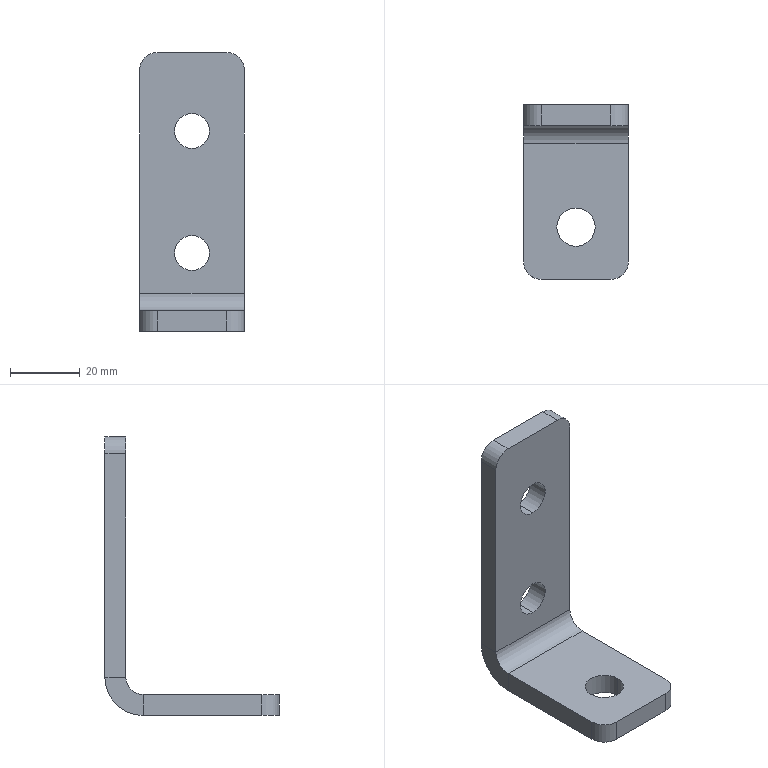Part | STEP file | SYL_0392D6J1SYL0380DJ100-808646 | 1 solid | 24 faces | box 30 x 50 x 80 mm | volume 20061 mm3 | cylinder 12 | plane 12 | commonest cylinder face diameters 10 x9 11 x2 22 x1
STEP:
#1=CARTESIAN_POINT('',(0.,25.,27.5));
#2=VERTEX_POINT('',#1);
#3=CARTESIAN_POINT('',(0.,19.,27.5));
#4=VERTEX_POINT('',#3);
#5=CARTESIAN_POINT('',(0.,19.,27.5));
#6=DIRECTION('',(0.,-1.,0.));
#7=VECTOR('',#6,1000.);
#8=LINE('',#5,#7);
#9=EDGE_CURVE('',#2,#4,#8,.T.);
#10=ORIENTED_EDGE('',*,*,#9,.F.);
#11=CARTESIAN_POINT('',(0.,25.,17.5));
#12=VERTEX_POINT('',#11);
#13=CARTESIAN_POINT('',(0.,25.,22.5));
#14=DIRECTION('',(0.,1.,0.));
#15=DIRECTION('',(0.,0.,1.));
#16=AXIS2_PLACEMENT_3D('',#13,#14,#15);
#17=CIRCLE('',#16,5.);
#18=EDGE_CURVE('',#2,#12,#17,.T.);
#19=ORIENTED_EDGE('',*,*,#18,.T.);
#20=CARTESIAN_POINT('',(0.,19.,17.5));
#21=VERTEX_POINT('',#20);
#22=CARTESIAN_POINT('',(0.,19.,17.5));
#23=DIRECTION('',(0.,-1.,0.));
#24=VECTOR('',#23,1000.);
#25=LINE('',#22,#24);
#26=EDGE_CURVE('',#12,#21,#25,.T.);
#27=ORIENTED_EDGE('',*,*,#26,.T.);
#28=CARTESIAN_POINT('',(0.,19.,22.5));
#29=DIRECTION('',(0.,1.,0.));
#30=DIRECTION('',(0.,0.,1.));
#31=AXIS2_PLACEMENT_3D('',#28,#29,#30);
#32=CIRCLE('',#31,5.);
#33=EDGE_CURVE('',#4,#21,#32,.T.);
#34=ORIENTED_EDGE('',*,*,#33,.F.);
#35=EDGE_LOOP('',(#10,#19,#27,#34));
#36=FACE_OUTER_BOUND('',#35,.T.);
#37=CARTESIAN_POINT('',(0.,19.,22.5));
#38=DIRECTION('',(0.,-1.,0.));
#39=DIRECTION('',(0.,0.,-1.));
#40=AXIS2_PLACEMENT_3D('',#37,#38,#39);
#41=CYLINDRICAL_SURFACE('',#40,5.);
#42=ADVANCED_FACE('',(#36),#41,.F.);
#43=CARTESIAN_POINT('',(0.,25.,62.5));
#44=VERTEX_POINT('',#43);
#45=CARTESIAN_POINT('',(0.,19.,62.5));
#46=VERTEX_POINT('',#45);
#47=CARTESIAN_POINT('',(0.,19.,62.5));
#48=DIRECTION('',(0.,-1.,0.));
#49=VECTOR('',#48,1000.);
#50=LINE('',#47,#49);
#51=EDGE_CURVE('',#44,#46,#50,.T.);
#52=ORIENTED_EDGE('',*,*,#51,.F.);
#53=CARTESIAN_POINT('',(0.,25.,52.5));
#54=VERTEX_POINT('',#53);
#55=CARTESIAN_POINT('',(0.,25.,57.5));
#56=DIRECTION('',(0.,1.,0.));
#57=DIRECTION('',(0.,0.,1.));
#58=AXIS2_PLACEMENT_3D('',#55,#56,#57);
#59=CIRCLE('',#58,5.);
#60=EDGE_CURVE('',#44,#54,#59,.T.);
#61=ORIENTED_EDGE('',*,*,#60,.T.);
#62=CARTESIAN_POINT('',(0.,19.,52.5));
#63=VERTEX_POINT('',#62);
#64=CARTESIAN_POINT('',(0.,19.,52.5));
#65=DIRECTION('',(0.,-1.,0.));
#66=VECTOR('',#65,1000.);
#67=LINE('',#64,#66);
#68=EDGE_CURVE('',#54,#63,#67,.T.);
#69=ORIENTED_EDGE('',*,*,#68,.T.);
#70=CARTESIAN_POINT('',(0.,19.,57.5));
#71=DIRECTION('',(0.,1.,0.));
#72=DIRECTION('',(0.,0.,1.));
#73=AXIS2_PLACEMENT_3D('',#70,#71,#72);
#74=CIRCLE('',#73,5.);
#75=EDGE_CURVE('',#46,#63,#74,.T.);
#76=ORIENTED_EDGE('',*,*,#75,.F.);
#77=EDGE_LOOP('',(#52,#61,#69,#76));
#78=FACE_OUTER_BOUND('',#77,.T.);
#79=CARTESIAN_POINT('',(0.,19.,57.5));
#80=DIRECTION('',(0.,-1.,0.));
#81=DIRECTION('',(0.,0.,-1.));
#82=AXIS2_PLACEMENT_3D('',#79,#80,#81);
#83=CYLINDRICAL_SURFACE('',#82,5.);
#84=ADVANCED_FACE('',(#78),#83,.F.);
#85=CARTESIAN_POINT('',(5.5,-10.,0.));
#86=VERTEX_POINT('',#85);
#87=CARTESIAN_POINT('',(5.5,-10.,6.));
#88=VERTEX_POINT('',#87);
#89=CARTESIAN_POINT('',(5.5,-10.,6.));
#90=DIRECTION('',(0.,0.,1.));
#91=VECTOR('',#90,1000.);
#92=LINE('',#89,#91);
#93=EDGE_CURVE('',#86,#88,#92,.T.);
#94=ORIENTED_EDGE('',*,*,#93,.F.);
#95=CARTESIAN_POINT('',(-5.5,-10.,0.));
#96=VERTEX_POINT('',#95);
#97=CARTESIAN_POINT('',(0.,-10.,0.));
#98=DIRECTION('',(0.,0.,-1.));
#99=DIRECTION('',(-1.,0.,0.));
#100=AXIS2_PLACEMENT_3D('',#97,#98,#99);
#101=CIRCLE('',#100,5.5);
#102=EDGE_CURVE('',#86,#96,#101,.T.);
#103=ORIENTED_EDGE('',*,*,#102,.T.);
#104=CARTESIAN_POINT('',(-5.5,-10.,6.));
#105=VERTEX_POINT('',#104);
#106=CARTESIAN_POINT('',(-5.5,-10.,6.));
#107=DIRECTION('',(0.,0.,1.));
#108=VECTOR('',#107,1000.);
#109=LINE('',#106,#108);
#110=EDGE_CURVE('',#96,#105,#109,.T.);
#111=ORIENTED_EDGE('',*,*,#110,.T.);
#112=CARTESIAN_POINT('',(0.,-10.,6.));
#113=DIRECTION('',(0.,0.,-1.));
#114=DIRECTION('',(1.,0.,0.));
#115=AXIS2_PLACEMENT_3D('',#112,#113,#114);
#116=CIRCLE('',#115,5.5);
#117=EDGE_CURVE('',#88,#105,#116,.T.);
#118=ORIENTED_EDGE('',*,*,#117,.F.);
#119=EDGE_LOOP('',(#94,#103,#111,#118));
#120=FACE_OUTER_BOUND('',#119,.T.);
#121=CARTESIAN_POINT('',(0.,-10.,6.));
#122=DIRECTION('',(0.,0.,1.));
#123=DIRECTION('',(1.,0.,0.));
#124=AXIS2_PLACEMENT_3D('',#121,#122,#123);
#125=CYLINDRICAL_SURFACE('',#124,5.5);
#126=ADVANCED_FACE('',(#120),#125,.F.);
#127=CARTESIAN_POINT('',(15.,25.,75.));
#128=VERTEX_POINT('',#127);
#129=CARTESIAN_POINT('',(15.,19.,75.));
#130=VERTEX_POINT('',#129);
#131=CARTESIAN_POINT('',(15.,19.,75.));
#132=DIRECTION('',(0.,-1.,0.));
#133=VECTOR('',#132,1000.);
#134=LINE('',#131,#133);
#135=EDGE_CURVE('',#128,#130,#134,.T.);
#136=ORIENTED_EDGE('',*,*,#135,.F.);
#137=CARTESIAN_POINT('',(10.,25.,80.));
#138=VERTEX_POINT('',#137);
#139=CARTESIAN_POINT('',(10.,25.,75.));
#140=DIRECTION('',(0.,-1.,0.));
#141=DIRECTION('',(0.,0.,-1.));
#142=AXIS2_PLACEMENT_3D('',#139,#140,#141);
#143=CIRCLE('',#142,5.);
#144=EDGE_CURVE('',#128,#138,#143,.T.);
#145=ORIENTED_EDGE('',*,*,#144,.T.);
#146=CARTESIAN_POINT('',(10.,19.,80.));
#147=VERTEX_POINT('',#146);
#148=CARTESIAN_POINT('',(10.,19.,80.));
#149=DIRECTION('',(0.,-1.,0.));
#150=VECTOR('',#149,1000.);
#151=LINE('',#148,#150);
#152=EDGE_CURVE('',#138,#147,#151,.T.);
#153=ORIENTED_EDGE('',*,*,#152,.T.);
#154=CARTESIAN_POINT('',(10.,19.,75.));
#155=DIRECTION('',(0.,-1.,0.));
#156=DIRECTION('',(1.,0.,0.));
#157=AXIS2_PLACEMENT_3D('',#154,#155,#156);
#158=CIRCLE('',#157,5.);
#159=EDGE_CURVE('',#130,#147,#158,.T.);
#160=ORIENTED_EDGE('',*,*,#159,.F.);
#161=EDGE_LOOP('',(#136,#145,#153,#160));
#162=FACE_OUTER_BOUND('',#161,.T.);
#163=CARTESIAN_POINT('',(10.,19.,75.));
#164=DIRECTION('',(0.,-1.,0.));
#165=DIRECTION('',(0.,0.,-1.));
#166=AXIS2_PLACEMENT_3D('',#163,#164,#165);
#167=CYLINDRICAL_SURFACE('',#166,5.);
#168=ADVANCED_FACE('',(#162),#167,.T.);
#169=ORIENTED_EDGE('',*,*,#152,.F.);
#170=CARTESIAN_POINT('',(-10.,25.,80.));
#171=VERTEX_POINT('',#170);
#172=CARTESIAN_POINT('',(7.872,25.,80.));
#173=DIRECTION('',(1.,0.,0.));
#174=VECTOR('',#173,1000.);
#175=LINE('',#172,#174);
#176=EDGE_CURVE('',#171,#138,#175,.T.);
#177=ORIENTED_EDGE('',*,*,#176,.F.);
#178=CARTESIAN_POINT('',(-10.,19.,80.));
#179=VERTEX_POINT('',#178);
#180=CARTESIAN_POINT('',(-10.,19.,80.));
#181=DIRECTION('',(0.,-1.,0.));
#182=VECTOR('',#181,1000.);
#183=LINE('',#180,#182);
#184=EDGE_CURVE('',#171,#179,#183,.T.);
#185=ORIENTED_EDGE('',*,*,#184,.T.);
#186=CARTESIAN_POINT('',(-10.,19.,80.));
#187=DIRECTION('',(1.,0.,0.));
#188=VECTOR('',#187,1000.);
#189=LINE('',#186,#188);
#190=EDGE_CURVE('',#179,#147,#189,.T.);
#191=ORIENTED_EDGE('',*,*,#190,.T.);
#192=EDGE_LOOP('',(#169,#177,#185,#191));
#193=FACE_OUTER_BOUND('',#192,.T.);
#194=CARTESIAN_POINT('',(-10.,19.,80.));
#195=DIRECTION('',(0.,0.,-1.));
#196=DIRECTION('',(1.,0.,0.));
#197=AXIS2_PLACEMENT_3D('',#194,#195,#196);
#198=PLANE('',#197);
#199=ADVANCED_FACE('',(#193),#198,.F.);
#200=ORIENTED_EDGE('',*,*,#184,.F.);
#201=CARTESIAN_POINT('',(-15.,25.,75.));
#202=VERTEX_POINT('',#201);
#203=CARTESIAN_POINT('',(-10.,25.,75.));
#204=DIRECTION('',(0.,-1.,0.));
#205=DIRECTION('',(0.,0.,-1.));
#206=AXIS2_PLACEMENT_3D('',#203,#204,#205);
#207=CIRCLE('',#206,5.);
#208=EDGE_CURVE('',#171,#202,#207,.T.);
#209=ORIENTED_EDGE('',*,*,#208,.T.);
#210=CARTESIAN_POINT('',(-15.,19.,75.));
#211=VERTEX_POINT('',#210);
#212=CARTESIAN_POINT('',(-15.,19.,75.));
#213=DIRECTION('',(0.,-1.,0.));
#214=VECTOR('',#213,1000.);
#215=LINE('',#212,#214);
#216=EDGE_CURVE('',#202,#211,#215,.T.);
#217=ORIENTED_EDGE('',*,*,#216,.T.);
#218=CARTESIAN_POINT('',(-10.,19.,75.));
#219=DIRECTION('',(0.,-1.,0.));
#220=DIRECTION('',(0.,0.,1.));
#221=AXIS2_PLACEMENT_3D('',#218,#219,#220);
#222=CIRCLE('',#221,5.);
#223=EDGE_CURVE('',#179,#211,#222,.T.);
#224=ORIENTED_EDGE('',*,*,#223,.F.);
#225=EDGE_LOOP('',(#200,#209,#217,#224));
#226=FACE_OUTER_BOUND('',#225,.T.);
#227=CARTESIAN_POINT('',(-10.,19.,75.));
#228=DIRECTION('',(0.,-1.,0.));
#229=DIRECTION('',(0.,0.,-1.));
#230=AXIS2_PLACEMENT_3D('',#227,#228,#229);
#231=CYLINDRICAL_SURFACE('',#230,5.);
#232=ADVANCED_FACE('',(#226),#231,.T.);
#233=ORIENTED_EDGE('',*,*,#216,.F.);
#234=CARTESIAN_POINT('',(-15.,25.,11.));
#235=VERTEX_POINT('',#234);
#236=CARTESIAN_POINT('',(-15.,25.,0.));
#237=DIRECTION('',(0.,0.,1.));
#238=VECTOR('',#237,1000.);
#239=LINE('',#236,#238);
#240=EDGE_CURVE('',#235,#202,#239,.T.);
#241=ORIENTED_EDGE('',*,*,#240,.F.);
#242=CARTESIAN_POINT('',(-15.,19.,11.));
#243=VERTEX_POINT('',#242);
#244=CARTESIAN_POINT('',(-15.,19.,11.));
#245=DIRECTION('',(0.,-1.,0.));
#246=VECTOR('',#245,1000.);
#247=LINE('',#244,#246);
#248=EDGE_CURVE('',#235,#243,#247,.T.);
#249=ORIENTED_EDGE('',*,*,#248,.T.);
#250=CARTESIAN_POINT('',(-15.,19.,11.));
#251=DIRECTION('',(0.,0.,1.));
#252=VECTOR('',#251,1000.);
#253=LINE('',#250,#252);
#254=EDGE_CURVE('',#243,#211,#253,.T.);
#255=ORIENTED_EDGE('',*,*,#254,.T.);
#256=EDGE_LOOP('',(#233,#241,#249,#255));
#257=FACE_OUTER_BOUND('',#256,.T.);
#258=CARTESIAN_POINT('',(-15.,19.,11.));
#259=DIRECTION('',(1.,0.,0.));
#260=DIRECTION('',(0.,0.,1.));
#261=AXIS2_PLACEMENT_3D('',#258,#259,#260);
#262=PLANE('',#261);
#263=ADVANCED_FACE('',(#257),#262,.F.);
#264=ORIENTED_EDGE('',*,*,#248,.F.);
#265=CARTESIAN_POINT('',(-15.,14.,0.));
#266=VERTEX_POINT('',#265);
#267=CARTESIAN_POINT('',(-15.,14.,11.));
#268=DIRECTION('',(1.,0.,0.));
#269=DIRECTION('',(0.,0.,1.));
#270=AXIS2_PLACEMENT_3D('',#267,#268,#269);
#271=CIRCLE('',#270,11.);
#272=EDGE_CURVE('',#266,#235,#271,.T.);
#273=ORIENTED_EDGE('',*,*,#272,.F.);
#274=CARTESIAN_POINT('',(-15.,14.,6.));
#275=VERTEX_POINT('',#274);
#276=CARTESIAN_POINT('',(-15.,14.,6.));
#277=DIRECTION('',(0.,0.,1.));
#278=VECTOR('',#277,1000.);
#279=LINE('',#276,#278);
#280=EDGE_CURVE('',#266,#275,#279,.T.);
#281=ORIENTED_EDGE('',*,*,#280,.T.);
#282=CARTESIAN_POINT('',(-15.,14.,11.));
#283=DIRECTION('',(1.,0.,0.));
#284=DIRECTION('',(0.,0.,-1.));
#285=AXIS2_PLACEMENT_3D('',#282,#283,#284);
#286=CIRCLE('',#285,5.);
#287=EDGE_CURVE('',#275,#243,#286,.T.);
#288=ORIENTED_EDGE('',*,*,#287,.T.);
#289=EDGE_LOOP('',(#264,#273,#281,#288));
#290=FACE_OUTER_BOUND('',#289,.T.);
#291=CARTESIAN_POINT('',(-15.,14.,11.));
#292=DIRECTION('',(-1.,0.,0.));
#293=DIRECTION('',(0.,0.,1.));
#294=AXIS2_PLACEMENT_3D('',#291,#292,#293);
#295=PLANE('',#294);
#296=ADVANCED_FACE('',(#290),#295,.T.);
#297=ORIENTED_EDGE('',*,*,#280,.F.);
#298=CARTESIAN_POINT('',(-15.,-20.,0.));
#299=VERTEX_POINT('',#298);
#300=CARTESIAN_POINT('',(-15.,0.,0.));
#301=DIRECTION('',(0.,1.,0.));
#302=VECTOR('',#301,1000.);
#303=LINE('',#300,#302);
#304=EDGE_CURVE('',#299,#266,#303,.T.);
#305=ORIENTED_EDGE('',*,*,#304,.F.);
#306=CARTESIAN_POINT('',(-15.,-20.,6.));
#307=VERTEX_POINT('',#306);
#308=CARTESIAN_POINT('',(-15.,-20.,6.));
#309=DIRECTION('',(0.,0.,1.));
#310=VECTOR('',#309,1000.);
#311=LINE('',#308,#310);
#312=EDGE_CURVE('',#299,#307,#311,.T.);
#313=ORIENTED_EDGE('',*,*,#312,.T.);
#314=CARTESIAN_POINT('',(-15.,-20.,6.));
#315=DIRECTION('',(0.,1.,0.));
#316=VECTOR('',#315,1000.);
#317=LINE('',#314,#316);
#318=EDGE_CURVE('',#307,#275,#317,.T.);
#319=ORIENTED_EDGE('',*,*,#318,.T.);
#320=EDGE_LOOP('',(#297,#305,#313,#319));
#321=FACE_OUTER_BOUND('',#320,.T.);
#322=CARTESIAN_POINT('',(-15.,-20.,6.));
#323=DIRECTION('',(1.,0.,0.));
#324=DIRECTION('',(0.,1.,0.));
#325=AXIS2_PLACEMENT_3D('',#322,#323,#324);
#326=PLANE('',#325);
#327=ADVANCED_FACE('',(#321),#326,.F.);
#328=ORIENTED_EDGE('',*,*,#312,.F.);
#329=CARTESIAN_POINT('',(-10.,-25.,0.));
#330=VERTEX_POINT('',#329);
#331=CARTESIAN_POINT('',(-10.,-20.,0.));
#332=DIRECTION('',(0.,0.,1.));
#333=DIRECTION('',(1.,0.,0.));
#334=AXIS2_PLACEMENT_3D('',#331,#332,#333);
#335=CIRCLE('',#334,5.);
#336=EDGE_CURVE('',#299,#330,#335,.T.);
#337=ORIENTED_EDGE('',*,*,#336,.T.);
#338=CARTESIAN_POINT('',(-10.,-25.,6.));
#339=VERTEX_POINT('',#338);
#340=CARTESIAN_POINT('',(-10.,-25.,6.));
#341=DIRECTION('',(0.,0.,1.));
#342=VECTOR('',#341,1000.);
#343=LINE('',#340,#342);
#344=EDGE_CURVE('',#330,#339,#343,.T.);
#345=ORIENTED_EDGE('',*,*,#344,.T.);
#346=CARTESIAN_POINT('',(-10.,-20.,6.));
#347=DIRECTION('',(0.,0.,1.));
#348=DIRECTION('',(-1.,0.,0.));
#349=AXIS2_PLACEMENT_3D('',#346,#347,#348);
#350=CIRCLE('',#349,5.);
#351=EDGE_CURVE('',#307,#339,#350,.T.);
#352=ORIENTED_EDGE('',*,*,#351,.F.);
#353=EDGE_LOOP('',(#328,#337,#345,#352));
#354=FACE_OUTER_BOUND('',#353,.T.);
#355=CARTESIAN_POINT('',(-10.,-20.,6.));
#356=DIRECTION('',(0.,0.,1.));
#357=DIRECTION('',(1.,0.,0.));
#358=AXIS2_PLACEMENT_3D('',#355,#356,#357);
#359=CYLINDRICAL_SURFACE('',#358,5.);
#360=ADVANCED_FACE('',(#354),#359,.T.);
#361=ORIENTED_EDGE('',*,*,#344,.F.);
#362=CARTESIAN_POINT('',(10.,-25.,0.));
#363=VERTEX_POINT('',#362);
#364=CARTESIAN_POINT('',(0.,-25.,0.));
#365=DIRECTION('',(-1.,0.,0.));
#366=VECTOR('',#365,1000.);
#367=LINE('',#364,#366);
#368=EDGE_CURVE('',#363,#330,#367,.T.);
#369=ORIENTED_EDGE('',*,*,#368,.F.);
#370=CARTESIAN_POINT('',(10.,-25.,6.));
#371=VERTEX_POINT('',#370);
#372=CARTESIAN_POINT('',(10.,-25.,6.));
#373=DIRECTION('',(0.,0.,1.));
#374=VECTOR('',#373,1000.);
#375=LINE('',#372,#374);
#376=EDGE_CURVE('',#363,#371,#375,.T.);
#377=ORIENTED_EDGE('',*,*,#376,.T.);
#378=CARTESIAN_POINT('',(10.,-25.,6.));
#379=DIRECTION('',(-1.,0.,0.));
#380=VECTOR('',#379,1000.);
#381=LINE('',#378,#380);
#382=EDGE_CURVE('',#371,#339,#381,.T.);
#383=ORIENTED_EDGE('',*,*,#382,.T.);
#384=EDGE_LOOP('',(#361,#369,#377,#383));
#385=FACE_OUTER_BOUND('',#384,.T.);
#386=CARTESIAN_POINT('',(10.,-25.,6.));
#387=DIRECTION('',(0.,1.,0.));
#388=DIRECTION('',(-1.,0.,0.));
#389=AXIS2_PLACEMENT_3D('',#386,#387,#388);
#390=PLANE('',#389);
#391=ADVANCED_FACE('',(#385),#390,.F.);
#392=ORIENTED_EDGE('',*,*,#376,.F.);
#393=CARTESIAN_POINT('',(15.,-20.,0.));
#394=VERTEX_POINT('',#393);
#395=CARTESIAN_POINT('',(10.,-20.,0.));
#396=DIRECTION('',(0.,0.,1.));
#397=DIRECTION('',(1.,0.,0.));
#398=AXIS2_PLACEMENT_3D('',#395,#396,#397);
#399=CIRCLE('',#398,5.);
#400=EDGE_CURVE('',#363,#394,#399,.T.);
#401=ORIENTED_EDGE('',*,*,#400,.T.);
#402=CARTESIAN_POINT('',(15.,-20.,6.));
#403=VERTEX_POINT('',#402);
#404=CARTESIAN_POINT('',(15.,-20.,6.));
#405=DIRECTION('',(0.,0.,1.));
#406=VECTOR('',#405,1000.);
#407=LINE('',#404,#406);
#408=EDGE_CURVE('',#394,#403,#407,.T.);
#409=ORIENTED_EDGE('',*,*,#408,.T.);
#410=CARTESIAN_POINT('',(10.,-20.,6.));
#411=DIRECTION('',(0.,0.,1.));
#412=DIRECTION('',(0.,-1.,0.));
#413=AXIS2_PLACEMENT_3D('',#410,#411,#412);
#414=CIRCLE('',#413,5.);
#415=EDGE_CURVE('',#371,#403,#414,.T.);
#416=ORIENTED_EDGE('',*,*,#415,.F.);
#417=EDGE_LOOP('',(#392,#401,#409,#416));
#418=FACE_OUTER_BOUND('',#417,.T.);
#419=CARTESIAN_POINT('',(10.,-20.,6.));
#420=DIRECTION('',(0.,0.,1.));
#421=DIRECTION('',(1.,0.,0.));
#422=AXIS2_PLACEMENT_3D('',#419,#420,#421);
#423=CYLINDRICAL_SURFACE('',#422,5.);
#424=ADVANCED_FACE('',(#418),#423,.T.);
#425=ORIENTED_EDGE('',*,*,#408,.F.);
#426=CARTESIAN_POINT('',(15.,14.,0.));
#427=VERTEX_POINT('',#426);
#428=CARTESIAN_POINT('',(15.,0.,0.));
#429=DIRECTION('',(0.,-1.,0.));
#430=VECTOR('',#429,1000.);
#431=LINE('',#428,#430);
#432=EDGE_CURVE('',#427,#394,#431,.T.);
#433=ORIENTED_EDGE('',*,*,#432,.F.);
#434=CARTESIAN_POINT('',(15.,14.,6.));
#435=VERTEX_POINT('',#434);
#436=CARTESIAN_POINT('',(15.,14.,6.));
#437=DIRECTION('',(0.,0.,1.));
#438=VECTOR('',#437,1000.);
#439=LINE('',#436,#438);
#440=EDGE_CURVE('',#427,#435,#439,.T.);
#441=ORIENTED_EDGE('',*,*,#440,.T.);
#442=CARTESIAN_POINT('',(15.,14.,6.));
#443=DIRECTION('',(0.,-1.,0.));
#444=VECTOR('',#443,1000.);
#445=LINE('',#442,#444);
#446=EDGE_CURVE('',#435,#403,#445,.T.);
#447=ORIENTED_EDGE('',*,*,#446,.T.);
#448=EDGE_LOOP('',(#425,#433,#441,#447));
#449=FACE_OUTER_BOUND('',#448,.T.);
#450=CARTESIAN_POINT('',(15.,14.,6.));
#451=DIRECTION('',(-1.,0.,0.));
#452=DIRECTION('',(0.,-1.,0.));
#453=AXIS2_PLACEMENT_3D('',#450,#451,#452);
#454=PLANE('',#453);
#455=ADVANCED_FACE('',(#449),#454,.F.);
#456=ORIENTED_EDGE('',*,*,#440,.F.);
#457=CARTESIAN_POINT('',(15.,25.,11.));
#458=VERTEX_POINT('',#457);
#459=CARTESIAN_POINT('',(15.,14.,11.));
#460=DIRECTION('',(-1.,0.,0.));
#461=DIRECTION('',(0.,0.,1.));
#462=AXIS2_PLACEMENT_3D('',#459,#460,#461);
#463=CIRCLE('',#462,11.);
#464=EDGE_CURVE('',#458,#427,#463,.T.);
#465=ORIENTED_EDGE('',*,*,#464,.F.);
#466=CARTESIAN_POINT('',(15.,19.,11.));
#467=VERTEX_POINT('',#466);
#468=CARTESIAN_POINT('',(15.,19.,11.));
#469=DIRECTION('',(0.,-1.,0.));
#470=VECTOR('',#469,1000.);
#471=LINE('',#468,#470);
#472=EDGE_CURVE('',#458,#467,#471,.T.);
#473=ORIENTED_EDGE('',*,*,#472,.T.);
#474=CARTESIAN_POINT('',(15.,14.,11.));
#475=DIRECTION('',(-1.,0.,0.));
#476=DIRECTION('',(0.,1.,0.));
#477=AXIS2_PLACEMENT_3D('',#474,#475,#476);
#478=CIRCLE('',#477,5.);
#479=EDGE_CURVE('',#467,#435,#478,.T.);
#480=ORIENTED_EDGE('',*,*,#479,.T.);
#481=EDGE_LOOP('',(#456,#465,#473,#480));
#482=FACE_OUTER_BOUND('',#481,.T.);
#483=CARTESIAN_POINT('',(15.,14.,11.));
#484=DIRECTION('',(1.,0.,0.));
#485=DIRECTION('',(0.,0.,-1.));
#486=AXIS2_PLACEMENT_3D('',#483,#484,#485);
#487=PLANE('',#486);
#488=ADVANCED_FACE('',(#482),#487,.T.);
#489=CARTESIAN_POINT('',(0.,25.,57.5));
#490=DIRECTION('',(0.,1.,0.));
#491=DIRECTION('',(0.,0.,1.));
#492=AXIS2_PLACEMENT_3D('',#489,#490,#491);
#493=CIRCLE('',#492,5.);
#494=EDGE_CURVE('',#54,#44,#493,.T.);
#495=ORIENTED_EDGE('',*,*,#494,.T.);
#496=ORIENTED_EDGE('',*,*,#51,.T.);
#497=CARTESIAN_POINT('',(0.,19.,57.5));
#498=DIRECTION('',(0.,1.,0.));
#499=DIRECTION('',(0.,0.,-1.));
#500=AXIS2_PLACEMENT_3D('',#497,#498,#499);
#501=CIRCLE('',#500,5.);
#502=EDGE_CURVE('',#63,#46,#501,.T.);
#503=ORIENTED_EDGE('',*,*,#502,.F.);
#504=ORIENTED_EDGE('',*,*,#68,.F.);
#505=EDGE_LOOP('',(#495,#496,#503,#504));
#506=FACE_OUTER_BOUND('',#505,.T.);
#507=CARTESIAN_POINT('',(0.,19.,57.5));
#508=DIRECTION('',(0.,-1.,0.));
#509=DIRECTION('',(0.,0.,-1.));
#510=AXIS2_PLACEMENT_3D('',#507,#508,#509);
#511=CYLINDRICAL_SURFACE('',#510,5.);
#512=ADVANCED_FACE('',(#506),#511,.F.);
#513=CARTESIAN_POINT('',(0.,25.,22.5));
#514=DIRECTION('',(0.,1.,0.));
#515=DIRECTION('',(0.,0.,1.));
#516=AXIS2_PLACEMENT_3D('',#513,#514,#515);
#517=CIRCLE('',#516,5.);
#518=EDGE_CURVE('',#12,#2,#517,.T.);
#519=ORIENTED_EDGE('',*,*,#518,.T.);
#520=ORIENTED_EDGE('',*,*,#9,.T.);
#521=CARTESIAN_POINT('',(0.,19.,22.5));
#522=DIRECTION('',(0.,1.,0.));
#523=DIRECTION('',(0.,0.,-1.));
#524=AXIS2_PLACEMENT_3D('',#521,#522,#523);
#525=CIRCLE('',#524,5.);
#526=EDGE_CURVE('',#21,#4,#525,.T.);
#527=ORIENTED_EDGE('',*,*,#526,.F.);
#528=ORIENTED_EDGE('',*,*,#26,.F.);
#529=EDGE_LOOP('',(#519,#520,#527,#528));
#530=FACE_OUTER_BOUND('',#529,.T.);
#531=CARTESIAN_POINT('',(0.,19.,22.5));
#532=DIRECTION('',(0.,-1.,0.));
#533=DIRECTION('',(0.,0.,-1.));
#534=AXIS2_PLACEMENT_3D('',#531,#532,#533);
#535=CYLINDRICAL_SURFACE('',#534,5.);
#536=ADVANCED_FACE('',(#530),#535,.F.);
#537=CARTESIAN_POINT('',(0.,-10.,0.));
#538=DIRECTION('',(0.,0.,-1.));
#539=DIRECTION('',(-1.,0.,0.));
#540=AXIS2_PLACEMENT_3D('',#537,#538,#539);
#541=CIRCLE('',#540,5.5);
#542=EDGE_CURVE('',#96,#86,#541,.T.);
#543=ORIENTED_EDGE('',*,*,#542,.T.);
#544=ORIENTED_EDGE('',*,*,#93,.T.);
#545=CARTESIAN_POINT('',(0.,-10.,6.));
#546=DIRECTION('',(0.,0.,-1.));
#547=DIRECTION('',(-1.,0.,0.));
#548=AXIS2_PLACEMENT_3D('',#545,#546,#547);
#549=CIRCLE('',#548,5.5);
#550=EDGE_CURVE('',#105,#88,#549,.T.);
#551=ORIENTED_EDGE('',*,*,#550,.F.);
#552=ORIENTED_EDGE('',*,*,#110,.F.);
#553=EDGE_LOOP('',(#543,#544,#551,#552));
#554=FACE_OUTER_BOUND('',#553,.T.);
#555=CARTESIAN_POINT('',(0.,-10.,6.));
#556=DIRECTION('',(0.,0.,1.));
#557=DIRECTION('',(1.,0.,0.));
#558=AXIS2_PLACEMENT_3D('',#555,#556,#557);
#559=CYLINDRICAL_SURFACE('',#558,5.5);
#560=ADVANCED_FACE('',(#554),#559,.F.);
#561=CARTESIAN_POINT('',(15.,25.,0.));
#562=DIRECTION('',(0.,0.,-1.));
#563=VECTOR('',#562,1000.);
#564=LINE('',#561,#563);
#565=EDGE_CURVE('',#128,#458,#564,.T.);
#566=ORIENTED_EDGE('',*,*,#565,.F.);
#567=ORIENTED_EDGE('',*,*,#135,.T.);
#568=CARTESIAN_POINT('',(15.,19.,75.));
#569=DIRECTION('',(0.,0.,-1.));
#570=VECTOR('',#569,1000.);
#571=LINE('',#568,#570);
#572=EDGE_CURVE('',#130,#467,#571,.T.);
#573=ORIENTED_EDGE('',*,*,#572,.T.);
#574=ORIENTED_EDGE('',*,*,#472,.F.);
#575=EDGE_LOOP('',(#566,#567,#573,#574));
#576=FACE_OUTER_BOUND('',#575,.T.);
#577=CARTESIAN_POINT('',(15.,19.,75.));
#578=DIRECTION('',(-1.,0.,0.));
#579=DIRECTION('',(0.,0.,-1.));
#580=AXIS2_PLACEMENT_3D('',#577,#578,#579);
#581=PLANE('',#580);
#582=ADVANCED_FACE('',(#576),#581,.F.);
#583=ORIENTED_EDGE('',*,*,#479,.F.);
#584=CARTESIAN_POINT('',(15.,19.,11.));
#585=DIRECTION('',(-1.,0.,0.));
#586=VECTOR('',#585,1000.);
#587=LINE('',#584,#586);
#588=EDGE_CURVE('',#467,#243,#587,.T.);
#589=ORIENTED_EDGE('',*,*,#588,.T.);
#590=ORIENTED_EDGE('',*,*,#287,.F.);
#591=CARTESIAN_POINT('',(-15.,14.,6.));
#592=DIRECTION('',(1.,0.,0.));
#593=VECTOR('',#592,1000.);
#594=LINE('',#591,#593);
#595=EDGE_CURVE('',#275,#435,#594,.T.);
#596=ORIENTED_EDGE('',*,*,#595,.T.);
#597=EDGE_LOOP('',(#583,#589,#590,#596));
#598=FACE_OUTER_BOUND('',#597,.T.);
#599=CARTESIAN_POINT('',(-15.,14.,11.));
#600=DIRECTION('',(-1.,0.,0.));
#601=DIRECTION('',(0.,0.,1.));
#602=AXIS2_PLACEMENT_3D('',#599,#600,#601);
#603=CYLINDRICAL_SURFACE('',#602,5.);
#604=ADVANCED_FACE('',(#598),#603,.F.);
#605=ORIENTED_EDGE('',*,*,#117,.T.);
#606=ORIENTED_EDGE('',*,*,#550,.T.);
#607=EDGE_LOOP('',(#605,#606));
#608=FACE_BOUND('',#607,.T.);
#609=ORIENTED_EDGE('',*,*,#415,.T.);
#610=ORIENTED_EDGE('',*,*,#446,.F.);
#611=ORIENTED_EDGE('',*,*,#595,.F.);
#612=ORIENTED_EDGE('',*,*,#318,.F.);
#613=ORIENTED_EDGE('',*,*,#351,.T.);
#614=ORIENTED_EDGE('',*,*,#382,.F.);
#615=EDGE_LOOP('',(#609,#610,#611,#612,#613,#614));
#616=FACE_OUTER_BOUND('',#615,.T.);
#617=CARTESIAN_POINT('',(0.,0.,6.));
#618=DIRECTION('',(0.,0.,1.));
#619=DIRECTION('',(1.,0.,0.));
#620=AXIS2_PLACEMENT_3D('',#617,#618,#619);
#621=PLANE('',#620);
#622=ADVANCED_FACE('',(#608,#616),#621,.T.);
#623=ORIENTED_EDGE('',*,*,#75,.T.);
#624=ORIENTED_EDGE('',*,*,#502,.T.);
#625=EDGE_LOOP('',(#623,#624));
#626=FACE_BOUND('',#625,.T.);
#627=ORIENTED_EDGE('',*,*,#33,.T.);
#628=ORIENTED_EDGE('',*,*,#526,.T.);
#629=EDGE_LOOP('',(#627,#628));
#630=FACE_BOUND('',#629,.T.);
#631=ORIENTED_EDGE('',*,*,#159,.T.);
#632=ORIENTED_EDGE('',*,*,#190,.F.);
#633=ORIENTED_EDGE('',*,*,#223,.T.);
#634=ORIENTED_EDGE('',*,*,#254,.F.);
#635=ORIENTED_EDGE('',*,*,#588,.F.);
#636=ORIENTED_EDGE('',*,*,#572,.F.);
#637=EDGE_LOOP('',(#631,#632,#633,#634,#635,#636));
#638=FACE_OUTER_BOUND('',#637,.T.);
#639=CARTESIAN_POINT('',(7.872,19.,0.));
#640=DIRECTION('',(0.,-1.,0.));
#641=DIRECTION('',(0.,0.,-1.));
#642=AXIS2_PLACEMENT_3D('',#639,#640,#641);
#643=PLANE('',#642);
#644=ADVANCED_FACE('',(#626,#630,#638),#643,.T.);
#645=ORIENTED_EDGE('',*,*,#464,.T.);
#646=CARTESIAN_POINT('',(-15.,14.,0.));
#647=DIRECTION('',(1.,0.,0.));
#648=VECTOR('',#647,1000.);
#649=LINE('',#646,#648);
#650=EDGE_CURVE('',#266,#427,#649,.T.);
#651=ORIENTED_EDGE('',*,*,#650,.F.);
#652=ORIENTED_EDGE('',*,*,#272,.T.);
#653=CARTESIAN_POINT('',(-15.,25.,11.));
#654=DIRECTION('',(-1.,0.,0.));
#655=VECTOR('',#654,1000.);
#656=LINE('',#653,#655);
#657=EDGE_CURVE('',#458,#235,#656,.T.);
#658=ORIENTED_EDGE('',*,*,#657,.F.);
#659=EDGE_LOOP('',(#645,#651,#652,#658));
#660=FACE_OUTER_BOUND('',#659,.T.);
#661=CARTESIAN_POINT('',(-15.,14.,11.));
#662=DIRECTION('',(-1.,0.,0.));
#663=DIRECTION('',(0.,0.,1.));
#664=AXIS2_PLACEMENT_3D('',#661,#662,#663);
#665=CYLINDRICAL_SURFACE('',#664,11.);
#666=ADVANCED_FACE('',(#660),#665,.T.);
#667=ORIENTED_EDGE('',*,*,#102,.F.);
#668=ORIENTED_EDGE('',*,*,#542,.F.);
#669=EDGE_LOOP('',(#667,#668));
#670=FACE_BOUND('',#669,.T.);
#671=ORIENTED_EDGE('',*,*,#400,.F.);
#672=ORIENTED_EDGE('',*,*,#368,.T.);
#673=ORIENTED_EDGE('',*,*,#336,.F.);
#674=ORIENTED_EDGE('',*,*,#304,.T.);
#675=ORIENTED_EDGE('',*,*,#650,.T.);
#676=ORIENTED_EDGE('',*,*,#432,.T.);
#677=EDGE_LOOP('',(#671,#672,#673,#674,#675,#676));
#678=FACE_OUTER_BOUND('',#677,.T.);
#679=CARTESIAN_POINT('',(0.,0.,0.));
#680=DIRECTION('',(0.,0.,1.));
#681=DIRECTION('',(1.,0.,0.));
#682=AXIS2_PLACEMENT_3D('',#679,#680,#681);
#683=PLANE('',#682);
#684=ADVANCED_FACE('',(#670,#678),#683,.F.);
#685=ORIENTED_EDGE('',*,*,#60,.F.);
#686=ORIENTED_EDGE('',*,*,#494,.F.);
#687=EDGE_LOOP('',(#685,#686));
#688=FACE_BOUND('',#687,.T.);
#689=ORIENTED_EDGE('',*,*,#18,.F.);
#690=ORIENTED_EDGE('',*,*,#518,.F.);
#691=EDGE_LOOP('',(#689,#690));
#692=FACE_BOUND('',#691,.T.);
#693=ORIENTED_EDGE('',*,*,#144,.F.);
#694=ORIENTED_EDGE('',*,*,#565,.T.);
#695=ORIENTED_EDGE('',*,*,#657,.T.);
#696=ORIENTED_EDGE('',*,*,#240,.T.);
#697=ORIENTED_EDGE('',*,*,#208,.F.);
#698=ORIENTED_EDGE('',*,*,#176,.T.);
#699=EDGE_LOOP('',(#693,#694,#695,#696,#697,#698));
#700=FACE_OUTER_BOUND('',#699,.T.);
#701=CARTESIAN_POINT('',(7.872,25.,0.));
#702=DIRECTION('',(0.,-1.,0.));
#703=DIRECTION('',(0.,0.,-1.));
#704=AXIS2_PLACEMENT_3D('',#701,#702,#703);
#705=PLANE('',#704);
#706=ADVANCED_FACE('',(#688,#692,#700),#705,.F.);
#707=CLOSED_SHELL('',(#42,#84,#126,#168,#199,#232,#263,#296,#327,#360,#391,#424,#455,#488,#512,#536,#560,#582,#604,#622,#644,#666,#684,#706));
#708=MANIFOLD_SOLID_BREP('',#707);
#709=CARTESIAN_POINT('',(0.,0.,0.));
#710=DIRECTION('',(0.,0.,1.));
#711=DIRECTION('',(1.,0.,0.));
#712=AXIS2_PLACEMENT_3D('',#709,#710,#711);
#713=(LENGTH_UNIT()NAMED_UNIT(*)SI_UNIT(.MILLI.,.METRE.));
#714=UNCERTAINTY_MEASURE_WITH_UNIT(LENGTH_MEASURE(0.00001),#713,'','');
#715=(NAMED_UNIT(*)PLANE_ANGLE_UNIT()SI_UNIT($,.RADIAN.));
#716=(NAMED_UNIT(*)SI_UNIT($,.STERADIAN.)SOLID_ANGLE_UNIT());
#717=(GEOMETRIC_REPRESENTATION_CONTEXT(3)GLOBAL_UNCERTAINTY_ASSIGNED_CONTEXT((#714))GLOBAL_UNIT_ASSIGNED_CONTEXT((#713,#715,#716))REPRESENTATION_CONTEXT('',''));
#718=ADVANCED_BREP_SHAPE_REPRESENTATION('',(#708,#712),#717);